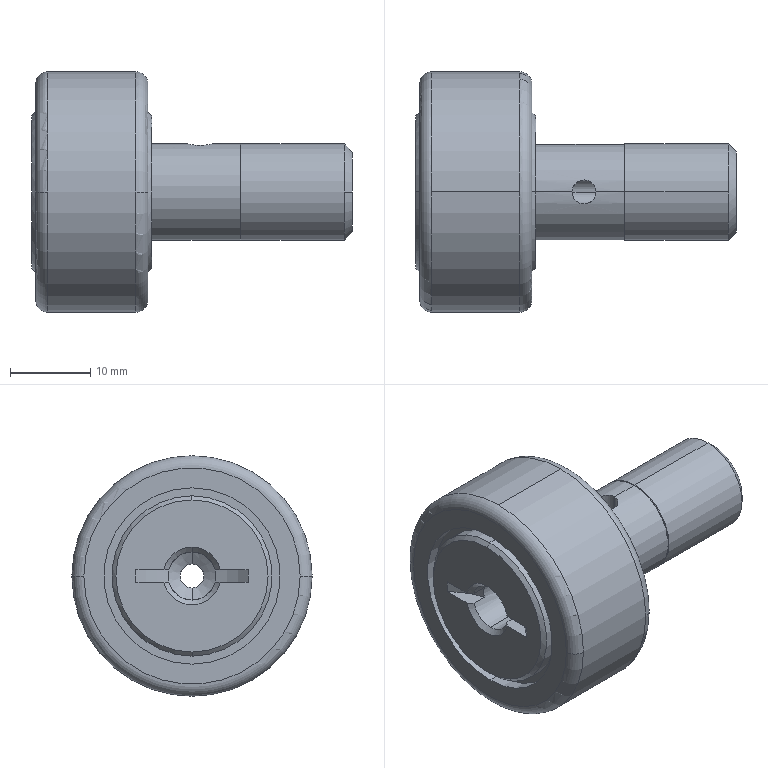Part | NX | 1 solid | 57 faces | box 40 x 30 x 30 mm | volume 12128 mm3 | cylinder 24 | cone 17 | plane 12 | torus 4 | commonest cylinder face diameters 20 x6 3 x4 6 x4 12 x4 22 x4 30 x2